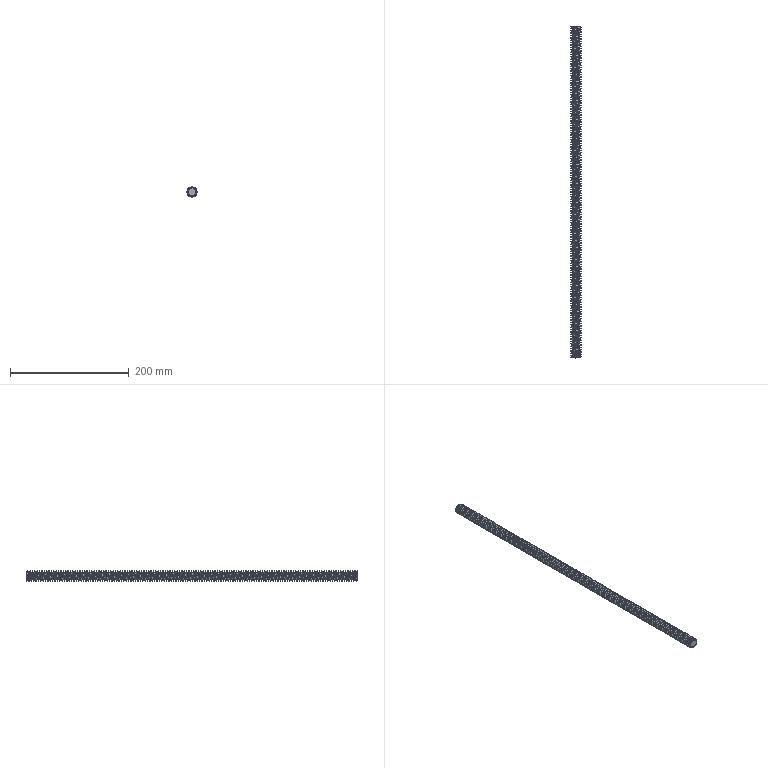Part | SolidWorks | features Extrusion 1, Helix 1, ICE 1, Sweep 1 | 1 solid | 286 faces | box 17 x 560 x 17 mm | volume 93030 mm3 | cylinder 281 | spline 3 | plane 2 | commonest cylinder face diameters 13 x281